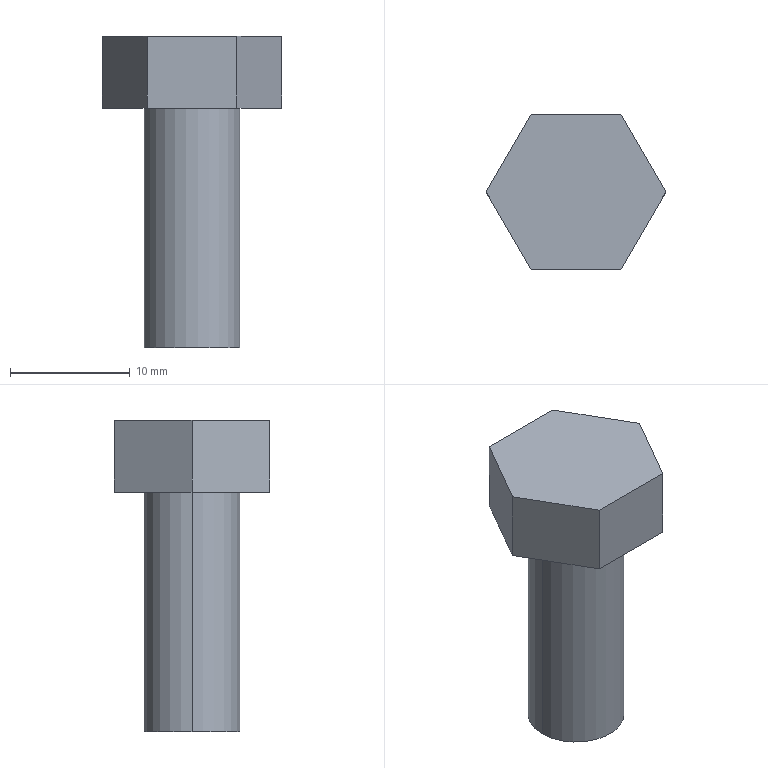Part | SolidWorks | features Extrusion 1, ICE 1 | 1 solid | 11 faces | box 15 x 12.99 x 26 mm | volume 1882 mm3 | plane 9 | cylinder 2 | commonest cylinder face diameters 8 x2
STEP:
#1=CARTESIAN_POINT('',(4.,0.,20.));
#2=VERTEX_POINT('',#1);
#3=CARTESIAN_POINT('',(-4.,0.,20.));
#4=VERTEX_POINT('',#3);
#5=CARTESIAN_POINT('',(0.,0.,20.));
#6=DIRECTION('',(0.,0.,1.));
#7=DIRECTION('',(1.,0.,0.));
#8=AXIS2_PLACEMENT_3D('',#5,#6,#7);
#9=CIRCLE('',#8,4.);
#10=EDGE_CURVE('',#2,#4,#9,.T.);
#11=ORIENTED_EDGE('',*,*,#10,.F.);
#12=CARTESIAN_POINT('',(4.,0.,0.));
#13=VERTEX_POINT('',#12);
#14=CARTESIAN_POINT('',(4.,0.,20.));
#15=DIRECTION('',(0.,0.,-1.));
#16=VECTOR('',#15,1000.);
#17=LINE('',#14,#16);
#18=EDGE_CURVE('',#2,#13,#17,.T.);
#19=ORIENTED_EDGE('',*,*,#18,.T.);
#20=CARTESIAN_POINT('',(-4.,0.,0.));
#21=VERTEX_POINT('',#20);
#22=CARTESIAN_POINT('',(0.,0.,0.));
#23=DIRECTION('',(0.,0.,1.));
#24=DIRECTION('',(1.,0.,0.));
#25=AXIS2_PLACEMENT_3D('',#22,#23,#24);
#26=CIRCLE('',#25,4.);
#27=EDGE_CURVE('',#13,#21,#26,.T.);
#28=ORIENTED_EDGE('',*,*,#27,.T.);
#29=CARTESIAN_POINT('',(-4.,0.,20.));
#30=DIRECTION('',(0.,0.,-1.));
#31=VECTOR('',#30,1000.);
#32=LINE('',#29,#31);
#33=EDGE_CURVE('',#4,#21,#32,.T.);
#34=ORIENTED_EDGE('',*,*,#33,.F.);
#35=EDGE_LOOP('',(#11,#19,#28,#34));
#36=FACE_OUTER_BOUND('',#35,.T.);
#37=CARTESIAN_POINT('',(0.,0.,20.));
#38=DIRECTION('',(0.,0.,-1.));
#39=DIRECTION('',(-1.,0.,0.));
#40=AXIS2_PLACEMENT_3D('',#37,#38,#39);
#41=CYLINDRICAL_SURFACE('',#40,4.);
#42=ADVANCED_FACE('',(#36),#41,.T.);
#43=ORIENTED_EDGE('',*,*,#18,.F.);
#44=CARTESIAN_POINT('',(0.,0.,20.));
#45=DIRECTION('',(0.,0.,1.));
#46=DIRECTION('',(1.,0.,0.));
#47=AXIS2_PLACEMENT_3D('',#44,#45,#46);
#48=CIRCLE('',#47,4.);
#49=EDGE_CURVE('',#4,#2,#48,.T.);
#50=ORIENTED_EDGE('',*,*,#49,.F.);
#51=ORIENTED_EDGE('',*,*,#33,.T.);
#52=CARTESIAN_POINT('',(0.,0.,0.));
#53=DIRECTION('',(0.,0.,1.));
#54=DIRECTION('',(1.,0.,0.));
#55=AXIS2_PLACEMENT_3D('',#52,#53,#54);
#56=CIRCLE('',#55,4.);
#57=EDGE_CURVE('',#21,#13,#56,.T.);
#58=ORIENTED_EDGE('',*,*,#57,.T.);
#59=EDGE_LOOP('',(#43,#50,#51,#58));
#60=FACE_OUTER_BOUND('',#59,.T.);
#61=CARTESIAN_POINT('',(0.,0.,20.));
#62=DIRECTION('',(0.,0.,-1.));
#63=DIRECTION('',(-1.,0.,0.));
#64=AXIS2_PLACEMENT_3D('',#61,#62,#63);
#65=CYLINDRICAL_SURFACE('',#64,4.);
#66=ADVANCED_FACE('',(#60),#65,.T.);
#67=ORIENTED_EDGE('',*,*,#57,.F.);
#68=ORIENTED_EDGE('',*,*,#27,.F.);
#69=EDGE_LOOP('',(#67,#68));
#70=FACE_OUTER_BOUND('',#69,.T.);
#71=CARTESIAN_POINT('',(0.,0.,0.));
#72=DIRECTION('',(0.,0.,1.));
#73=DIRECTION('',(1.,0.,0.));
#74=AXIS2_PLACEMENT_3D('',#71,#72,#73);
#75=PLANE('',#74);
#76=ADVANCED_FACE('',(#70),#75,.F.);
#77=CARTESIAN_POINT('',(3.75,6.495,20.));
#78=VERTEX_POINT('',#77);
#79=CARTESIAN_POINT('',(-3.75,6.495,20.));
#80=VERTEX_POINT('',#79);
#81=CARTESIAN_POINT('',(3.75,6.495,20.));
#82=DIRECTION('',(-1.,0.,0.));
#83=VECTOR('',#82,1000.);
#84=LINE('',#81,#83);
#85=EDGE_CURVE('',#78,#80,#84,.T.);
#86=ORIENTED_EDGE('',*,*,#85,.T.);
#87=CARTESIAN_POINT('',(-3.75,6.495,26.));
#88=VERTEX_POINT('',#87);
#89=CARTESIAN_POINT('',(-3.75,6.495,26.));
#90=DIRECTION('',(0.,0.,-1.));
#91=VECTOR('',#90,1000.);
#92=LINE('',#89,#91);
#93=EDGE_CURVE('',#88,#80,#92,.T.);
#94=ORIENTED_EDGE('',*,*,#93,.F.);
#95=CARTESIAN_POINT('',(3.75,6.495,26.));
#96=VERTEX_POINT('',#95);
#97=CARTESIAN_POINT('',(3.75,6.495,26.));
#98=DIRECTION('',(-1.,0.,0.));
#99=VECTOR('',#98,1000.);
#100=LINE('',#97,#99);
#101=EDGE_CURVE('',#96,#88,#100,.T.);
#102=ORIENTED_EDGE('',*,*,#101,.F.);
#103=CARTESIAN_POINT('',(3.75,6.495,26.));
#104=DIRECTION('',(0.,0.,-1.));
#105=VECTOR('',#104,1000.);
#106=LINE('',#103,#105);
#107=EDGE_CURVE('',#96,#78,#106,.T.);
#108=ORIENTED_EDGE('',*,*,#107,.T.);
#109=EDGE_LOOP('',(#86,#94,#102,#108));
#110=FACE_OUTER_BOUND('',#109,.T.);
#111=CARTESIAN_POINT('',(3.75,6.495,26.));
#112=DIRECTION('',(0.,-1.,0.));
#113=DIRECTION('',(1.,0.,0.));
#114=AXIS2_PLACEMENT_3D('',#111,#112,#113);
#115=PLANE('',#114);
#116=ADVANCED_FACE('',(#110),#115,.F.);
#117=CARTESIAN_POINT('',(-7.5,0.,20.));
#118=VERTEX_POINT('',#117);
#119=CARTESIAN_POINT('',(-3.75,6.495,20.));
#120=DIRECTION('',(-0.5,-0.866,0.));
#121=VECTOR('',#120,1000.);
#122=LINE('',#119,#121);
#123=EDGE_CURVE('',#80,#118,#122,.T.);
#124=ORIENTED_EDGE('',*,*,#123,.T.);
#125=CARTESIAN_POINT('',(-7.5,0.,26.));
#126=VERTEX_POINT('',#125);
#127=CARTESIAN_POINT('',(-7.5,0.,26.));
#128=DIRECTION('',(0.,0.,-1.));
#129=VECTOR('',#128,1000.);
#130=LINE('',#127,#129);
#131=EDGE_CURVE('',#126,#118,#130,.T.);
#132=ORIENTED_EDGE('',*,*,#131,.F.);
#133=CARTESIAN_POINT('',(-3.75,6.495,26.));
#134=DIRECTION('',(-0.5,-0.866,0.));
#135=VECTOR('',#134,1000.);
#136=LINE('',#133,#135);
#137=EDGE_CURVE('',#88,#126,#136,.T.);
#138=ORIENTED_EDGE('',*,*,#137,.F.);
#139=ORIENTED_EDGE('',*,*,#93,.T.);
#140=EDGE_LOOP('',(#124,#132,#138,#139));
#141=FACE_OUTER_BOUND('',#140,.T.);
#142=CARTESIAN_POINT('',(-3.75,6.495,26.));
#143=DIRECTION('',(0.866,-0.5,0.));
#144=DIRECTION('',(0.5,0.866,0.));
#145=AXIS2_PLACEMENT_3D('',#142,#143,#144);
#146=PLANE('',#145);
#147=ADVANCED_FACE('',(#141),#146,.F.);
#148=CARTESIAN_POINT('',(-3.75,-6.495,20.));
#149=VERTEX_POINT('',#148);
#150=CARTESIAN_POINT('',(-7.5,0.,20.));
#151=DIRECTION('',(0.5,-0.866,0.));
#152=VECTOR('',#151,1000.);
#153=LINE('',#150,#152);
#154=EDGE_CURVE('',#118,#149,#153,.T.);
#155=ORIENTED_EDGE('',*,*,#154,.T.);
#156=CARTESIAN_POINT('',(-3.75,-6.495,26.));
#157=VERTEX_POINT('',#156);
#158=CARTESIAN_POINT('',(-3.75,-6.495,26.));
#159=DIRECTION('',(0.,0.,-1.));
#160=VECTOR('',#159,1000.);
#161=LINE('',#158,#160);
#162=EDGE_CURVE('',#157,#149,#161,.T.);
#163=ORIENTED_EDGE('',*,*,#162,.F.);
#164=CARTESIAN_POINT('',(-7.5,0.,26.));
#165=DIRECTION('',(0.5,-0.866,0.));
#166=VECTOR('',#165,1000.);
#167=LINE('',#164,#166);
#168=EDGE_CURVE('',#126,#157,#167,.T.);
#169=ORIENTED_EDGE('',*,*,#168,.F.);
#170=ORIENTED_EDGE('',*,*,#131,.T.);
#171=EDGE_LOOP('',(#155,#163,#169,#170));
#172=FACE_OUTER_BOUND('',#171,.T.);
#173=CARTESIAN_POINT('',(-7.5,0.,26.));
#174=DIRECTION('',(0.866,0.5,0.));
#175=DIRECTION('',(-0.5,0.866,0.));
#176=AXIS2_PLACEMENT_3D('',#173,#174,#175);
#177=PLANE('',#176);
#178=ADVANCED_FACE('',(#172),#177,.F.);
#179=CARTESIAN_POINT('',(3.75,-6.495,20.));
#180=VERTEX_POINT('',#179);
#181=CARTESIAN_POINT('',(-3.75,-6.495,20.));
#182=DIRECTION('',(1.,0.,0.));
#183=VECTOR('',#182,1000.);
#184=LINE('',#181,#183);
#185=EDGE_CURVE('',#149,#180,#184,.T.);
#186=ORIENTED_EDGE('',*,*,#185,.T.);
#187=CARTESIAN_POINT('',(3.75,-6.495,26.));
#188=VERTEX_POINT('',#187);
#189=CARTESIAN_POINT('',(3.75,-6.495,26.));
#190=DIRECTION('',(0.,0.,-1.));
#191=VECTOR('',#190,1000.);
#192=LINE('',#189,#191);
#193=EDGE_CURVE('',#188,#180,#192,.T.);
#194=ORIENTED_EDGE('',*,*,#193,.F.);
#195=CARTESIAN_POINT('',(-3.75,-6.495,26.));
#196=DIRECTION('',(1.,0.,0.));
#197=VECTOR('',#196,1000.);
#198=LINE('',#195,#197);
#199=EDGE_CURVE('',#157,#188,#198,.T.);
#200=ORIENTED_EDGE('',*,*,#199,.F.);
#201=ORIENTED_EDGE('',*,*,#162,.T.);
#202=EDGE_LOOP('',(#186,#194,#200,#201));
#203=FACE_OUTER_BOUND('',#202,.T.);
#204=CARTESIAN_POINT('',(-3.75,-6.495,26.));
#205=DIRECTION('',(0.,1.,0.));
#206=DIRECTION('',(-1.,0.,0.));
#207=AXIS2_PLACEMENT_3D('',#204,#205,#206);
#208=PLANE('',#207);
#209=ADVANCED_FACE('',(#203),#208,.F.);
#210=CARTESIAN_POINT('',(7.5,0.,20.));
#211=VERTEX_POINT('',#210);
#212=CARTESIAN_POINT('',(3.75,-6.495,20.));
#213=DIRECTION('',(0.5,0.866,0.));
#214=VECTOR('',#213,1000.);
#215=LINE('',#212,#214);
#216=EDGE_CURVE('',#180,#211,#215,.T.);
#217=ORIENTED_EDGE('',*,*,#216,.T.);
#218=CARTESIAN_POINT('',(7.5,0.,26.));
#219=VERTEX_POINT('',#218);
#220=CARTESIAN_POINT('',(7.5,0.,26.));
#221=DIRECTION('',(0.,0.,-1.));
#222=VECTOR('',#221,1000.);
#223=LINE('',#220,#222);
#224=EDGE_CURVE('',#219,#211,#223,.T.);
#225=ORIENTED_EDGE('',*,*,#224,.F.);
#226=CARTESIAN_POINT('',(3.75,-6.495,26.));
#227=DIRECTION('',(0.5,0.866,0.));
#228=VECTOR('',#227,1000.);
#229=LINE('',#226,#228);
#230=EDGE_CURVE('',#188,#219,#229,.T.);
#231=ORIENTED_EDGE('',*,*,#230,.F.);
#232=ORIENTED_EDGE('',*,*,#193,.T.);
#233=EDGE_LOOP('',(#217,#225,#231,#232));
#234=FACE_OUTER_BOUND('',#233,.T.);
#235=CARTESIAN_POINT('',(3.75,-6.495,26.));
#236=DIRECTION('',(-0.866,0.5,0.));
#237=DIRECTION('',(-0.5,-0.866,0.));
#238=AXIS2_PLACEMENT_3D('',#235,#236,#237);
#239=PLANE('',#238);
#240=ADVANCED_FACE('',(#234),#239,.F.);
#241=CARTESIAN_POINT('',(7.5,0.,20.));
#242=DIRECTION('',(-0.5,0.866,0.));
#243=VECTOR('',#242,1000.);
#244=LINE('',#241,#243);
#245=EDGE_CURVE('',#211,#78,#244,.T.);
#246=ORIENTED_EDGE('',*,*,#245,.T.);
#247=ORIENTED_EDGE('',*,*,#107,.F.);
#248=CARTESIAN_POINT('',(7.5,0.,26.));
#249=DIRECTION('',(-0.5,0.866,0.));
#250=VECTOR('',#249,1000.);
#251=LINE('',#248,#250);
#252=EDGE_CURVE('',#219,#96,#251,.T.);
#253=ORIENTED_EDGE('',*,*,#252,.F.);
#254=ORIENTED_EDGE('',*,*,#224,.T.);
#255=EDGE_LOOP('',(#246,#247,#253,#254));
#256=FACE_OUTER_BOUND('',#255,.T.);
#257=CARTESIAN_POINT('',(7.5,0.,26.));
#258=DIRECTION('',(-0.866,-0.5,0.));
#259=DIRECTION('',(0.5,-0.866,0.));
#260=AXIS2_PLACEMENT_3D('',#257,#258,#259);
#261=PLANE('',#260);
#262=ADVANCED_FACE('',(#256),#261,.F.);
#263=ORIENTED_EDGE('',*,*,#101,.T.);
#264=ORIENTED_EDGE('',*,*,#137,.T.);
#265=ORIENTED_EDGE('',*,*,#168,.T.);
#266=ORIENTED_EDGE('',*,*,#199,.T.);
#267=ORIENTED_EDGE('',*,*,#230,.T.);
#268=ORIENTED_EDGE('',*,*,#252,.T.);
#269=EDGE_LOOP('',(#263,#264,#265,#266,#267,#268));
#270=FACE_OUTER_BOUND('',#269,.T.);
#271=CARTESIAN_POINT('',(0.,0.,26.));
#272=DIRECTION('',(0.,0.,1.));
#273=DIRECTION('',(1.,0.,0.));
#274=AXIS2_PLACEMENT_3D('',#271,#272,#273);
#275=PLANE('',#274);
#276=ADVANCED_FACE('',(#270),#275,.T.);
#277=ORIENTED_EDGE('',*,*,#49,.T.);
#278=ORIENTED_EDGE('',*,*,#10,.T.);
#279=EDGE_LOOP('',(#277,#278));
#280=FACE_BOUND('',#279,.T.);
#281=ORIENTED_EDGE('',*,*,#85,.F.);
#282=ORIENTED_EDGE('',*,*,#245,.F.);
#283=ORIENTED_EDGE('',*,*,#216,.F.);
#284=ORIENTED_EDGE('',*,*,#185,.F.);
#285=ORIENTED_EDGE('',*,*,#154,.F.);
#286=ORIENTED_EDGE('',*,*,#123,.F.);
#287=EDGE_LOOP('',(#281,#282,#283,#284,#285,#286));
#288=FACE_OUTER_BOUND('',#287,.T.);
#289=CARTESIAN_POINT('',(0.,0.,20.));
#290=DIRECTION('',(0.,0.,1.));
#291=DIRECTION('',(1.,0.,0.));
#292=AXIS2_PLACEMENT_3D('',#289,#290,#291);
#293=PLANE('',#292);
#294=ADVANCED_FACE('',(#280,#288),#293,.F.);
#295=CLOSED_SHELL('',(#42,#66,#76,#116,#147,#178,#209,#240,#262,#276,#294));
#296=MANIFOLD_SOLID_BREP('',#295);
#297=CARTESIAN_POINT('',(0.,0.,0.));
#298=DIRECTION('',(0.,0.,1.));
#299=DIRECTION('',(1.,0.,0.));
#300=AXIS2_PLACEMENT_3D('',#297,#298,#299);
#301=(LENGTH_UNIT()NAMED_UNIT(*)SI_UNIT(.MILLI.,.METRE.));
#302=UNCERTAINTY_MEASURE_WITH_UNIT(LENGTH_MEASURE(0.00001),#301,'','');
#303=(NAMED_UNIT(*)PLANE_ANGLE_UNIT()SI_UNIT($,.RADIAN.));
#304=(NAMED_UNIT(*)SI_UNIT($,.STERADIAN.)SOLID_ANGLE_UNIT());
#305=(GEOMETRIC_REPRESENTATION_CONTEXT(3)GLOBAL_UNCERTAINTY_ASSIGNED_CONTEXT((#302))GLOBAL_UNIT_ASSIGNED_CONTEXT((#301,#303,#304))REPRESENTATION_CONTEXT('',''));
#306=ADVANCED_BREP_SHAPE_REPRESENTATION('',(#296,#300),#305);